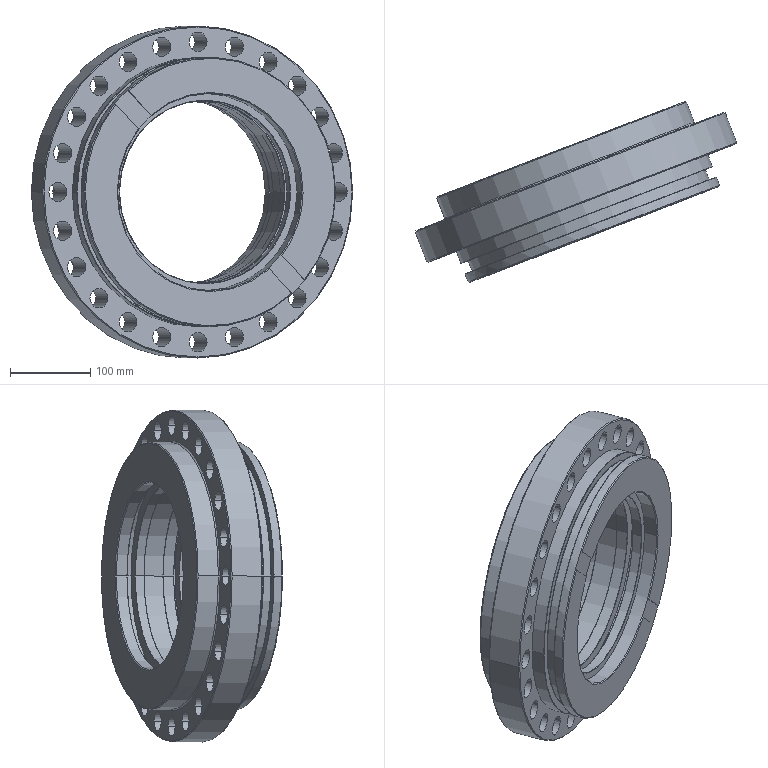Part | SolidWorks | features BaseBody 1, Scale 1 | 1 solid | 132 faces | box 400.613 x 225.724 x 414 mm | volume 6404045 mm3 | cylinder 74 | spline 26 | plane 18 | cone 14 | commonest cylinder face diameters 24 x48 228 x6 256.8 x4 336 x4 228.48 x2 234 x2